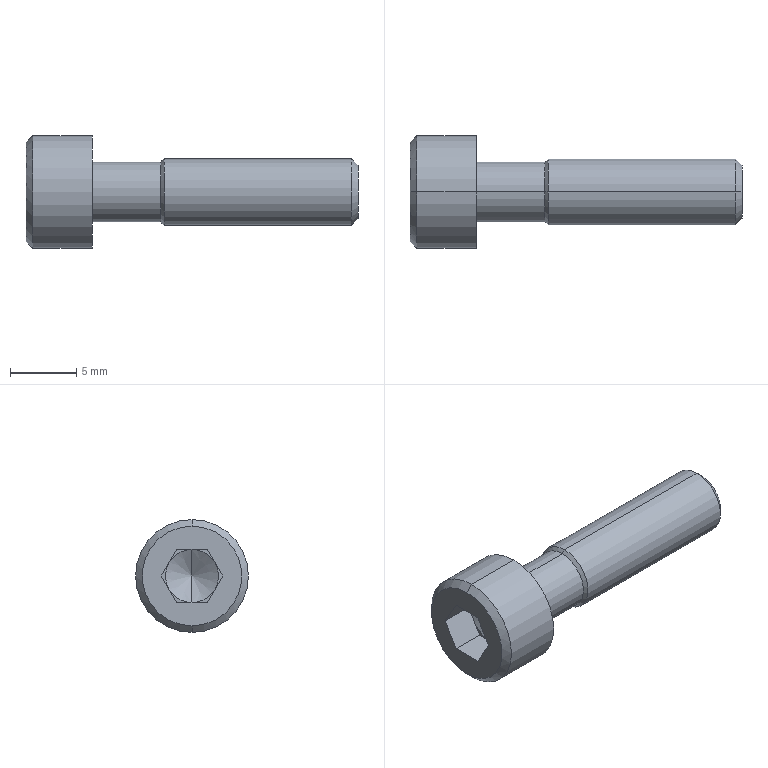Part | STEP file | 0232_Z_SCBS5-20_1 | 1 solid | 29 faces | box 25 x 8.5 x 8.5 mm | volume 612.597 mm3 | plane 15 | cone 8 | cylinder 6 | commonest cylinder face diameters 4.509 x2 5 x2 8.5 x2